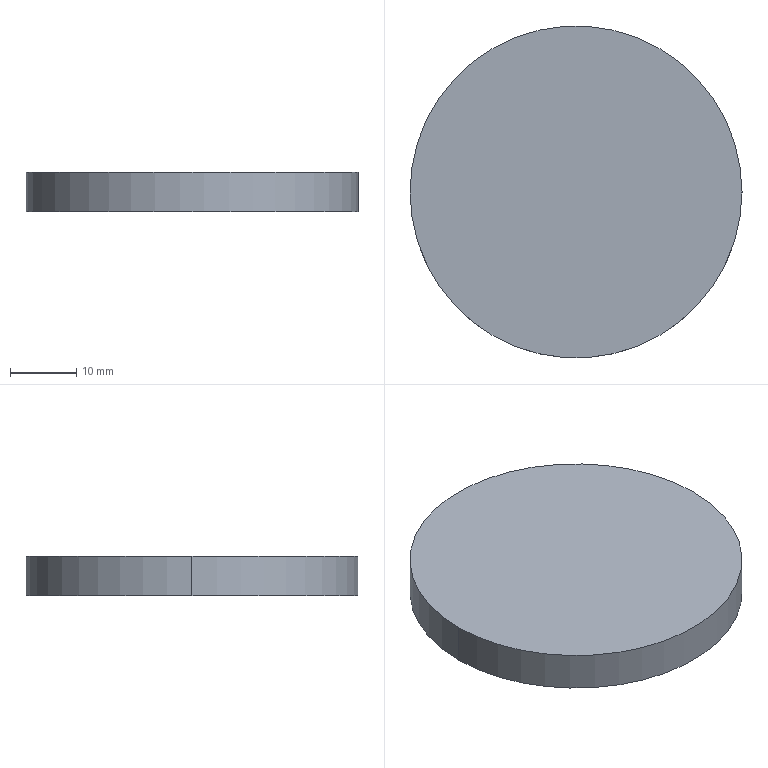Part | SolidWorks | features Extrusion 1 | 1 solid | 4 faces | box 50 x 50 x 6 mm | volume 11781 mm3 | cylinder 2 | plane 2 | commonest cylinder face diameters 50 x2
STEP:
#1=CARTESIAN_POINT('',(25.,0.,6.));
#2=VERTEX_POINT('',#1);
#3=CARTESIAN_POINT('',(-25.,0.,6.));
#4=VERTEX_POINT('',#3);
#5=CARTESIAN_POINT('',(0.,0.,6.));
#6=DIRECTION('',(0.,0.,1.));
#7=DIRECTION('',(1.,0.,0.));
#8=AXIS2_PLACEMENT_3D('',#5,#6,#7);
#9=CIRCLE('',#8,25.);
#10=EDGE_CURVE('',#2,#4,#9,.T.);
#11=ORIENTED_EDGE('',*,*,#10,.F.);
#12=CARTESIAN_POINT('',(25.,0.,0.));
#13=VERTEX_POINT('',#12);
#14=CARTESIAN_POINT('',(25.,0.,6.));
#15=DIRECTION('',(0.,0.,-1.));
#16=VECTOR('',#15,1000.);
#17=LINE('',#14,#16);
#18=EDGE_CURVE('',#2,#13,#17,.T.);
#19=ORIENTED_EDGE('',*,*,#18,.T.);
#20=CARTESIAN_POINT('',(-25.,0.,0.));
#21=VERTEX_POINT('',#20);
#22=CARTESIAN_POINT('',(0.,0.,0.));
#23=DIRECTION('',(0.,0.,1.));
#24=DIRECTION('',(1.,0.,0.));
#25=AXIS2_PLACEMENT_3D('',#22,#23,#24);
#26=CIRCLE('',#25,25.);
#27=EDGE_CURVE('',#13,#21,#26,.T.);
#28=ORIENTED_EDGE('',*,*,#27,.T.);
#29=CARTESIAN_POINT('',(-25.,0.,6.));
#30=DIRECTION('',(0.,0.,-1.));
#31=VECTOR('',#30,1000.);
#32=LINE('',#29,#31);
#33=EDGE_CURVE('',#4,#21,#32,.T.);
#34=ORIENTED_EDGE('',*,*,#33,.F.);
#35=EDGE_LOOP('',(#11,#19,#28,#34));
#36=FACE_OUTER_BOUND('',#35,.T.);
#37=CARTESIAN_POINT('',(0.,0.,6.));
#38=DIRECTION('',(0.,0.,-1.));
#39=DIRECTION('',(-1.,0.,0.));
#40=AXIS2_PLACEMENT_3D('',#37,#38,#39);
#41=CYLINDRICAL_SURFACE('',#40,25.);
#42=ADVANCED_FACE('',(#36),#41,.T.);
#43=ORIENTED_EDGE('',*,*,#18,.F.);
#44=CARTESIAN_POINT('',(0.,0.,6.));
#45=DIRECTION('',(0.,0.,1.));
#46=DIRECTION('',(1.,0.,0.));
#47=AXIS2_PLACEMENT_3D('',#44,#45,#46);
#48=CIRCLE('',#47,25.);
#49=EDGE_CURVE('',#4,#2,#48,.T.);
#50=ORIENTED_EDGE('',*,*,#49,.F.);
#51=ORIENTED_EDGE('',*,*,#33,.T.);
#52=CARTESIAN_POINT('',(0.,0.,0.));
#53=DIRECTION('',(0.,0.,1.));
#54=DIRECTION('',(1.,0.,0.));
#55=AXIS2_PLACEMENT_3D('',#52,#53,#54);
#56=CIRCLE('',#55,25.);
#57=EDGE_CURVE('',#21,#13,#56,.T.);
#58=ORIENTED_EDGE('',*,*,#57,.T.);
#59=EDGE_LOOP('',(#43,#50,#51,#58));
#60=FACE_OUTER_BOUND('',#59,.T.);
#61=CARTESIAN_POINT('',(0.,0.,6.));
#62=DIRECTION('',(0.,0.,-1.));
#63=DIRECTION('',(-1.,0.,0.));
#64=AXIS2_PLACEMENT_3D('',#61,#62,#63);
#65=CYLINDRICAL_SURFACE('',#64,25.);
#66=ADVANCED_FACE('',(#60),#65,.T.);
#67=ORIENTED_EDGE('',*,*,#49,.T.);
#68=ORIENTED_EDGE('',*,*,#10,.T.);
#69=EDGE_LOOP('',(#67,#68));
#70=FACE_OUTER_BOUND('',#69,.T.);
#71=CARTESIAN_POINT('',(0.,0.,6.));
#72=DIRECTION('',(0.,0.,1.));
#73=DIRECTION('',(1.,0.,0.));
#74=AXIS2_PLACEMENT_3D('',#71,#72,#73);
#75=PLANE('',#74);
#76=ADVANCED_FACE('',(#70),#75,.T.);
#77=ORIENTED_EDGE('',*,*,#57,.F.);
#78=ORIENTED_EDGE('',*,*,#27,.F.);
#79=EDGE_LOOP('',(#77,#78));
#80=FACE_OUTER_BOUND('',#79,.T.);
#81=CARTESIAN_POINT('',(0.,0.,0.));
#82=DIRECTION('',(0.,0.,1.));
#83=DIRECTION('',(1.,0.,0.));
#84=AXIS2_PLACEMENT_3D('',#81,#82,#83);
#85=PLANE('',#84);
#86=ADVANCED_FACE('',(#80),#85,.F.);
#87=CLOSED_SHELL('',(#42,#66,#76,#86));
#88=MANIFOLD_SOLID_BREP('',#87);
#89=CARTESIAN_POINT('',(0.,0.,0.));
#90=DIRECTION('',(0.,0.,1.));
#91=DIRECTION('',(1.,0.,0.));
#92=AXIS2_PLACEMENT_3D('',#89,#90,#91);
#93=(LENGTH_UNIT()NAMED_UNIT(*)SI_UNIT(.MILLI.,.METRE.));
#94=UNCERTAINTY_MEASURE_WITH_UNIT(LENGTH_MEASURE(0.00001),#93,'','');
#95=(NAMED_UNIT(*)PLANE_ANGLE_UNIT()SI_UNIT($,.RADIAN.));
#96=(NAMED_UNIT(*)SI_UNIT($,.STERADIAN.)SOLID_ANGLE_UNIT());
#97=(GEOMETRIC_REPRESENTATION_CONTEXT(3)GLOBAL_UNCERTAINTY_ASSIGNED_CONTEXT((#94))GLOBAL_UNIT_ASSIGNED_CONTEXT((#93,#95,#96))REPRESENTATION_CONTEXT('',''));
#98=ADVANCED_BREP_SHAPE_REPRESENTATION('',(#88,#92),#97);